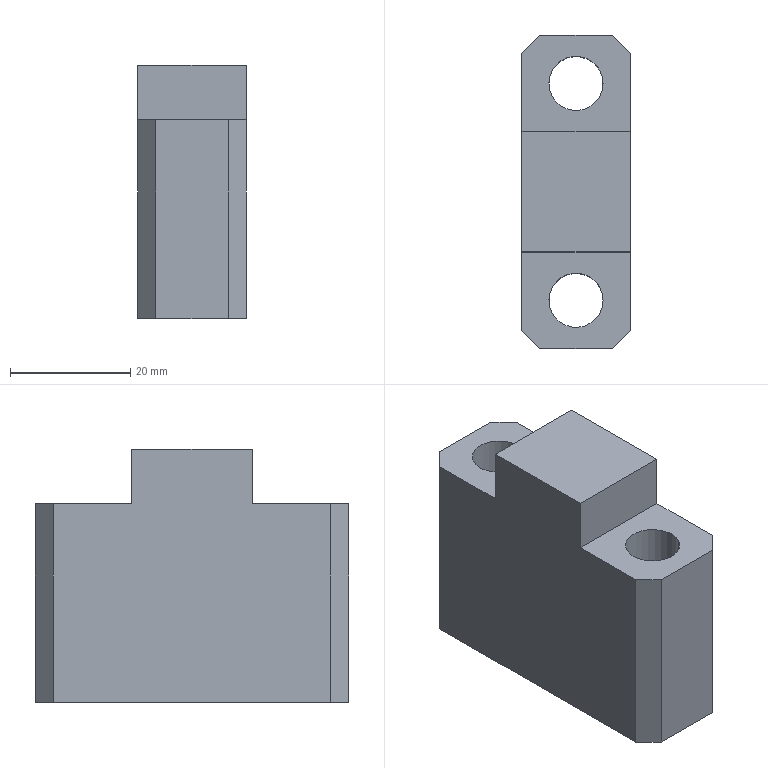Part | CATIA | 1 solid | 18 faces | box 18 x 52 x 42 mm | volume 29335 mm3 | plane 14 | cylinder 4 | commonest cylinder face diameters 9 x4
STEP:
#1=CARTESIAN_POINT('',(-1312.,219.5,-9.));
#2=VERTEX_POINT('',#1);
#3=CARTESIAN_POINT('',(-1312.,219.5,-42.));
#4=VERTEX_POINT('',#3);
#5=CARTESIAN_POINT('',(-1312.,219.5,-21.));
#6=DIRECTION('',(0.,0.,-1.));
#7=VECTOR('',#6,1.);
#8=LINE('',#5,#7);
#9=EDGE_CURVE('',#2,#4,#8,.T.);
#10=ORIENTED_EDGE('',*,*,#9,.T.);
#11=CARTESIAN_POINT('',(-1315.,222.5,-42.));
#12=VERTEX_POINT('',#11);
#13=CARTESIAN_POINT('',(-1313.5,221.,-42.));
#14=DIRECTION('',(-0.7071,0.7071,0.));
#15=VECTOR('',#14,1.);
#16=LINE('',#13,#15);
#17=EDGE_CURVE('',#4,#12,#16,.T.);
#18=ORIENTED_EDGE('',*,*,#17,.T.);
#19=CARTESIAN_POINT('',(-1315.,222.5,-9.));
#20=VERTEX_POINT('',#19);
#21=CARTESIAN_POINT('',(-1315.,222.5,-21.));
#22=DIRECTION('',(0.,0.,-1.));
#23=VECTOR('',#22,1.);
#24=LINE('',#21,#23);
#25=EDGE_CURVE('',#20,#12,#24,.T.);
#26=ORIENTED_EDGE('',*,*,#25,.F.);
#27=CARTESIAN_POINT('',(-1313.5,221.,-9.));
#28=DIRECTION('',(-0.7071,0.7071,0.));
#29=VECTOR('',#28,1.);
#30=LINE('',#27,#29);
#31=EDGE_CURVE('',#20,#2,#30,.F.);
#32=ORIENTED_EDGE('',*,*,#31,.T.);
#33=EDGE_LOOP('',(#10,#18,#26,#32));
#34=FACE_OUTER_BOUND('',#33,.T.);
#35=CARTESIAN_POINT('',(-1312.,219.5,8.4));
#36=DIRECTION('',(0.7071,0.7071,0.));
#37=DIRECTION('',(0.,0.,-1.));
#38=AXIS2_PLACEMENT_3D('',#35,#36,#37);
#39=PLANE('',#38);
#40=ADVANCED_FACE('',(#34),#39,.T.);
#41=CARTESIAN_POINT('',(-1330.,186.5,0.));
#42=VERTEX_POINT('',#41);
#43=CARTESIAN_POINT('',(-1312.,186.5,0.));
#44=VERTEX_POINT('',#43);
#45=CARTESIAN_POINT('',(-1321.,186.5,0.));
#46=DIRECTION('',(1.,0.,0.));
#47=VECTOR('',#46,1.);
#48=LINE('',#45,#47);
#49=EDGE_CURVE('',#42,#44,#48,.T.);
#50=ORIENTED_EDGE('',*,*,#49,.T.);
#51=CARTESIAN_POINT('',(-1312.,206.5,0.));
#52=VERTEX_POINT('',#51);
#53=CARTESIAN_POINT('',(-1312.,196.5,0.));
#54=DIRECTION('',(0.,1.,0.));
#55=VECTOR('',#54,1.);
#56=LINE('',#53,#55);
#57=EDGE_CURVE('',#44,#52,#56,.T.);
#58=ORIENTED_EDGE('',*,*,#57,.T.);
#59=CARTESIAN_POINT('',(-1330.,206.5,0.));
#60=VERTEX_POINT('',#59);
#61=CARTESIAN_POINT('',(-1321.,206.5,0.));
#62=DIRECTION('',(1.,0.,0.));
#63=VECTOR('',#62,1.);
#64=LINE('',#61,#63);
#65=EDGE_CURVE('',#60,#52,#64,.T.);
#66=ORIENTED_EDGE('',*,*,#65,.F.);
#67=CARTESIAN_POINT('',(-1330.,196.5,0.));
#68=DIRECTION('',(0.,-1.,0.));
#69=VECTOR('',#68,1.);
#70=LINE('',#67,#69);
#71=EDGE_CURVE('',#60,#42,#70,.T.);
#72=ORIENTED_EDGE('',*,*,#71,.T.);
#73=EDGE_LOOP('',(#50,#58,#66,#72));
#74=FACE_OUTER_BOUND('',#73,.T.);
#75=CARTESIAN_POINT('',(0.,0.,0.));
#76=DIRECTION('',(0.,0.,1.));
#77=DIRECTION('',(1.,0.,0.));
#78=AXIS2_PLACEMENT_3D('',#75,#76,#77);
#79=PLANE('',#78);
#80=ADVANCED_FACE('',(#74),#79,.T.);
#81=CARTESIAN_POINT('',(-1312.,186.5,-9.));
#82=VERTEX_POINT('',#81);
#83=CARTESIAN_POINT('',(-1312.,186.5,-4.5));
#84=DIRECTION('',(0.,0.,1.));
#85=VECTOR('',#84,1.);
#86=LINE('',#83,#85);
#87=EDGE_CURVE('',#82,#44,#86,.T.);
#88=ORIENTED_EDGE('',*,*,#87,.F.);
#89=CARTESIAN_POINT('',(-1312.,173.5,-9.));
#90=VERTEX_POINT('',#89);
#91=CARTESIAN_POINT('',(-1312.,180.,-9.));
#92=DIRECTION('',(0.,-1.,0.));
#93=VECTOR('',#92,1.);
#94=LINE('',#91,#93);
#95=EDGE_CURVE('',#82,#90,#94,.T.);
#96=ORIENTED_EDGE('',*,*,#95,.T.);
#97=CARTESIAN_POINT('',(-1312.,173.5,-42.));
#98=VERTEX_POINT('',#97);
#99=CARTESIAN_POINT('',(-1312.,173.5,-25.5));
#100=DIRECTION('',(0.,0.,1.));
#101=VECTOR('',#100,1.);
#102=LINE('',#99,#101);
#103=EDGE_CURVE('',#90,#98,#102,.F.);
#104=ORIENTED_EDGE('',*,*,#103,.T.);
#105=CARTESIAN_POINT('',(-1312.,196.5,-42.));
#106=DIRECTION('',(0.,1.,0.));
#107=VECTOR('',#106,1.);
#108=LINE('',#105,#107);
#109=EDGE_CURVE('',#98,#4,#108,.T.);
#110=ORIENTED_EDGE('',*,*,#109,.T.);
#111=ORIENTED_EDGE('',*,*,#9,.F.);
#112=CARTESIAN_POINT('',(-1312.,206.5,-9.));
#113=VERTEX_POINT('',#112);
#114=CARTESIAN_POINT('',(-1312.,213.,-9.));
#115=DIRECTION('',(0.,1.,0.));
#116=VECTOR('',#115,1.);
#117=LINE('',#114,#116);
#118=EDGE_CURVE('',#113,#2,#117,.T.);
#119=ORIENTED_EDGE('',*,*,#118,.F.);
#120=CARTESIAN_POINT('',(-1312.,206.5,-4.5));
#121=DIRECTION('',(0.,0.,1.));
#122=VECTOR('',#121,1.);
#123=LINE('',#120,#122);
#124=EDGE_CURVE('',#113,#52,#123,.T.);
#125=ORIENTED_EDGE('',*,*,#124,.T.);
#126=ORIENTED_EDGE('',*,*,#57,.F.);
#127=EDGE_LOOP('',(#88,#96,#104,#110,#111,#119,#125,#126));
#128=FACE_OUTER_BOUND('',#127,.T.);
#129=CARTESIAN_POINT('',(-1312.,170.5,0.));
#130=DIRECTION('',(-1.,0.,0.));
#131=DIRECTION('',(0.,1.,0.));
#132=AXIS2_PLACEMENT_3D('',#129,#130,#131);
#133=PLANE('',#132);
#134=ADVANCED_FACE('',(#128),#133,.F.);
#135=ORIENTED_EDGE('',*,*,#25,.T.);
#136=CARTESIAN_POINT('',(-1327.,222.5,-42.));
#137=VERTEX_POINT('',#136);
#138=CARTESIAN_POINT('',(-1321.,222.5,-42.));
#139=DIRECTION('',(1.,0.,0.));
#140=VECTOR('',#139,1.);
#141=LINE('',#138,#140);
#142=EDGE_CURVE('',#137,#12,#141,.T.);
#143=ORIENTED_EDGE('',*,*,#142,.F.);
#144=CARTESIAN_POINT('',(-1327.,222.5,-9.));
#145=VERTEX_POINT('',#144);
#146=CARTESIAN_POINT('',(-1327.,222.5,-25.5));
#147=DIRECTION('',(0.,0.,1.));
#148=VECTOR('',#147,1.);
#149=LINE('',#146,#148);
#150=EDGE_CURVE('',#145,#137,#149,.F.);
#151=ORIENTED_EDGE('',*,*,#150,.F.);
#152=CARTESIAN_POINT('',(-1321.,222.5,-9.));
#153=DIRECTION('',(1.,0.,0.));
#154=VECTOR('',#153,1.);
#155=LINE('',#152,#154);
#156=EDGE_CURVE('',#145,#20,#155,.T.);
#157=ORIENTED_EDGE('',*,*,#156,.T.);
#158=EDGE_LOOP('',(#135,#143,#151,#157));
#159=FACE_OUTER_BOUND('',#158,.T.);
#160=CARTESIAN_POINT('',(-1330.,222.5,0.));
#161=DIRECTION('',(0.,1.,0.));
#162=DIRECTION('',(1.,0.,0.));
#163=AXIS2_PLACEMENT_3D('',#160,#161,#162);
#164=PLANE('',#163);
#165=ADVANCED_FACE('',(#159),#164,.T.);
#166=CARTESIAN_POINT('',(-1315.,170.5,-9.));
#167=VERTEX_POINT('',#166);
#168=CARTESIAN_POINT('',(-1315.,170.5,-42.));
#169=VERTEX_POINT('',#168);
#170=CARTESIAN_POINT('',(-1315.,170.5,-21.));
#171=DIRECTION('',(0.,0.,1.));
#172=VECTOR('',#171,1.);
#173=LINE('',#170,#172);
#174=EDGE_CURVE('',#167,#169,#173,.F.);
#175=ORIENTED_EDGE('',*,*,#174,.T.);
#176=CARTESIAN_POINT('',(-1313.5,172.,-42.));
#177=DIRECTION('',(-0.7071,-0.7071,0.));
#178=VECTOR('',#177,1.);
#179=LINE('',#176,#178);
#180=EDGE_CURVE('',#169,#98,#179,.F.);
#181=ORIENTED_EDGE('',*,*,#180,.T.);
#182=ORIENTED_EDGE('',*,*,#103,.F.);
#183=CARTESIAN_POINT('',(-1313.5,172.,-9.));
#184=DIRECTION('',(-0.7071,-0.7071,0.));
#185=VECTOR('',#184,1.);
#186=LINE('',#183,#185);
#187=EDGE_CURVE('',#167,#90,#186,.F.);
#188=ORIENTED_EDGE('',*,*,#187,.F.);
#189=EDGE_LOOP('',(#175,#181,#182,#188));
#190=FACE_OUTER_BOUND('',#189,.T.);
#191=CARTESIAN_POINT('',(-1312.,173.5,-50.4));
#192=DIRECTION('',(0.7071,-0.7071,0.));
#193=DIRECTION('',(0.,0.,1.));
#194=AXIS2_PLACEMENT_3D('',#191,#192,#193);
#195=PLANE('',#194);
#196=ADVANCED_FACE('',(#190),#195,.T.);
#197=CARTESIAN_POINT('',(-1327.,170.5,-9.));
#198=VERTEX_POINT('',#197);
#199=CARTESIAN_POINT('',(-1327.,170.5,-42.));
#200=VERTEX_POINT('',#199);
#201=CARTESIAN_POINT('',(-1327.,170.5,-25.5));
#202=DIRECTION('',(0.,0.,-1.));
#203=VECTOR('',#202,1.);
#204=LINE('',#201,#203);
#205=EDGE_CURVE('',#198,#200,#204,.T.);
#206=ORIENTED_EDGE('',*,*,#205,.T.);
#207=CARTESIAN_POINT('',(-1321.,170.5,-42.));
#208=DIRECTION('',(-1.,0.,0.));
#209=VECTOR('',#208,1.);
#210=LINE('',#207,#209);
#211=EDGE_CURVE('',#169,#200,#210,.T.);
#212=ORIENTED_EDGE('',*,*,#211,.F.);
#213=ORIENTED_EDGE('',*,*,#174,.F.);
#214=CARTESIAN_POINT('',(-1321.,170.5,-9.));
#215=DIRECTION('',(-1.,0.,0.));
#216=VECTOR('',#215,1.);
#217=LINE('',#214,#216);
#218=EDGE_CURVE('',#167,#198,#217,.T.);
#219=ORIENTED_EDGE('',*,*,#218,.T.);
#220=EDGE_LOOP('',(#206,#212,#213,#219));
#221=FACE_OUTER_BOUND('',#220,.T.);
#222=CARTESIAN_POINT('',(-1312.,170.5,0.));
#223=DIRECTION('',(0.,-1.,0.));
#224=DIRECTION('',(-1.,0.,0.));
#225=AXIS2_PLACEMENT_3D('',#222,#223,#224);
#226=PLANE('',#225);
#227=ADVANCED_FACE('',(#221),#226,.T.);
#228=ORIENTED_EDGE('',*,*,#150,.T.);
#229=CARTESIAN_POINT('',(-1330.,219.5,-42.));
#230=VERTEX_POINT('',#229);
#231=CARTESIAN_POINT('',(-1328.5,221.,-42.));
#232=DIRECTION('',(0.7071,0.7071,0.));
#233=VECTOR('',#232,1.);
#234=LINE('',#231,#233);
#235=EDGE_CURVE('',#137,#230,#234,.F.);
#236=ORIENTED_EDGE('',*,*,#235,.T.);
#237=CARTESIAN_POINT('',(-1330.,219.5,-9.));
#238=VERTEX_POINT('',#237);
#239=CARTESIAN_POINT('',(-1330.,219.5,-21.));
#240=DIRECTION('',(0.,0.,1.));
#241=VECTOR('',#240,1.);
#242=LINE('',#239,#241);
#243=EDGE_CURVE('',#238,#230,#242,.F.);
#244=ORIENTED_EDGE('',*,*,#243,.F.);
#245=CARTESIAN_POINT('',(-1328.5,221.,-9.));
#246=DIRECTION('',(0.7071,0.7071,0.));
#247=VECTOR('',#246,1.);
#248=LINE('',#245,#247);
#249=EDGE_CURVE('',#145,#238,#248,.F.);
#250=ORIENTED_EDGE('',*,*,#249,.F.);
#251=EDGE_LOOP('',(#228,#236,#244,#250));
#252=FACE_OUTER_BOUND('',#251,.T.);
#253=CARTESIAN_POINT('',(-1330.,219.5,-50.4));
#254=DIRECTION('',(-0.7071,0.7071,0.));
#255=DIRECTION('',(0.,0.,1.));
#256=AXIS2_PLACEMENT_3D('',#253,#254,#255);
#257=PLANE('',#256);
#258=ADVANCED_FACE('',(#252),#257,.T.);
#259=ORIENTED_EDGE('',*,*,#71,.F.);
#260=CARTESIAN_POINT('',(-1330.,206.5,-9.));
#261=VERTEX_POINT('',#260);
#262=CARTESIAN_POINT('',(-1330.,206.5,-4.5));
#263=DIRECTION('',(0.,0.,1.));
#264=VECTOR('',#263,1.);
#265=LINE('',#262,#264);
#266=EDGE_CURVE('',#261,#60,#265,.T.);
#267=ORIENTED_EDGE('',*,*,#266,.F.);
#268=CARTESIAN_POINT('',(-1330.,213.,-9.));
#269=DIRECTION('',(0.,1.,0.));
#270=VECTOR('',#269,1.);
#271=LINE('',#268,#270);
#272=EDGE_CURVE('',#261,#238,#271,.T.);
#273=ORIENTED_EDGE('',*,*,#272,.T.);
#274=ORIENTED_EDGE('',*,*,#243,.T.);
#275=CARTESIAN_POINT('',(-1330.,173.5,-42.));
#276=VERTEX_POINT('',#275);
#277=CARTESIAN_POINT('',(-1330.,196.5,-42.));
#278=DIRECTION('',(0.,-1.,0.));
#279=VECTOR('',#278,1.);
#280=LINE('',#277,#279);
#281=EDGE_CURVE('',#230,#276,#280,.T.);
#282=ORIENTED_EDGE('',*,*,#281,.T.);
#283=CARTESIAN_POINT('',(-1330.,173.5,-9.));
#284=VERTEX_POINT('',#283);
#285=CARTESIAN_POINT('',(-1330.,173.5,-25.5));
#286=DIRECTION('',(0.,0.,-1.));
#287=VECTOR('',#286,1.);
#288=LINE('',#285,#287);
#289=EDGE_CURVE('',#284,#276,#288,.T.);
#290=ORIENTED_EDGE('',*,*,#289,.F.);
#291=CARTESIAN_POINT('',(-1330.,186.5,-9.));
#292=VERTEX_POINT('',#291);
#293=CARTESIAN_POINT('',(-1330.,180.,-9.));
#294=DIRECTION('',(0.,-1.,0.));
#295=VECTOR('',#294,1.);
#296=LINE('',#293,#295);
#297=EDGE_CURVE('',#292,#284,#296,.T.);
#298=ORIENTED_EDGE('',*,*,#297,.F.);
#299=CARTESIAN_POINT('',(-1330.,186.5,-4.5));
#300=DIRECTION('',(0.,0.,1.));
#301=VECTOR('',#300,1.);
#302=LINE('',#299,#301);
#303=EDGE_CURVE('',#292,#42,#302,.T.);
#304=ORIENTED_EDGE('',*,*,#303,.T.);
#305=EDGE_LOOP('',(#259,#267,#273,#274,#282,#290,#298,#304));
#306=FACE_OUTER_BOUND('',#305,.T.);
#307=CARTESIAN_POINT('',(-1330.,222.5,0.));
#308=DIRECTION('',(1.,0.,0.));
#309=DIRECTION('',(0.,-1.,0.));
#310=AXIS2_PLACEMENT_3D('',#307,#308,#309);
#311=PLANE('',#310);
#312=ADVANCED_FACE('',(#306),#311,.F.);
#313=ORIENTED_EDGE('',*,*,#289,.T.);
#314=CARTESIAN_POINT('',(-1328.5,172.,-42.));
#315=DIRECTION('',(0.7071,-0.7071,0.));
#316=VECTOR('',#315,1.);
#317=LINE('',#314,#316);
#318=EDGE_CURVE('',#276,#200,#317,.T.);
#319=ORIENTED_EDGE('',*,*,#318,.T.);
#320=ORIENTED_EDGE('',*,*,#205,.F.);
#321=CARTESIAN_POINT('',(-1328.5,172.,-9.));
#322=DIRECTION('',(0.7071,-0.7071,0.));
#323=VECTOR('',#322,1.);
#324=LINE('',#321,#323);
#325=EDGE_CURVE('',#198,#284,#324,.F.);
#326=ORIENTED_EDGE('',*,*,#325,.T.);
#327=EDGE_LOOP('',(#313,#319,#320,#326));
#328=FACE_OUTER_BOUND('',#327,.T.);
#329=CARTESIAN_POINT('',(-1330.,173.5,8.4));
#330=DIRECTION('',(-0.7071,-0.7071,0.));
#331=DIRECTION('',(0.,0.,-1.));
#332=AXIS2_PLACEMENT_3D('',#329,#330,#331);
#333=PLANE('',#332);
#334=ADVANCED_FACE('',(#328),#333,.T.);
#335=ORIENTED_EDGE('',*,*,#87,.T.);
#336=ORIENTED_EDGE('',*,*,#49,.F.);
#337=ORIENTED_EDGE('',*,*,#303,.F.);
#338=CARTESIAN_POINT('',(-1321.,186.5,-9.));
#339=DIRECTION('',(1.,0.,0.));
#340=VECTOR('',#339,1.);
#341=LINE('',#338,#340);
#342=EDGE_CURVE('',#82,#292,#341,.F.);
#343=ORIENTED_EDGE('',*,*,#342,.F.);
#344=EDGE_LOOP('',(#335,#336,#337,#343));
#345=FACE_OUTER_BOUND('',#344,.T.);
#346=CARTESIAN_POINT('',(-1405.,186.5,0.));
#347=DIRECTION('',(0.,1.,0.));
#348=DIRECTION('',(1.,0.,0.));
#349=AXIS2_PLACEMENT_3D('',#346,#347,#348);
#350=PLANE('',#349);
#351=ADVANCED_FACE('',(#345),#350,.F.);
#352=ORIENTED_EDGE('',*,*,#266,.T.);
#353=ORIENTED_EDGE('',*,*,#65,.T.);
#354=ORIENTED_EDGE('',*,*,#124,.F.);
#355=CARTESIAN_POINT('',(-1321.,206.5,-9.));
#356=DIRECTION('',(-1.,0.,0.));
#357=VECTOR('',#356,1.);
#358=LINE('',#355,#357);
#359=EDGE_CURVE('',#261,#113,#358,.F.);
#360=ORIENTED_EDGE('',*,*,#359,.F.);
#361=EDGE_LOOP('',(#352,#353,#354,#360));
#362=FACE_OUTER_BOUND('',#361,.T.);
#363=CARTESIAN_POINT('',(-1159.802,206.5,0.));
#364=DIRECTION('',(0.,-1.,0.));
#365=DIRECTION('',(-1.,0.,0.));
#366=AXIS2_PLACEMENT_3D('',#363,#364,#365);
#367=PLANE('',#366);
#368=ADVANCED_FACE('',(#362),#367,.F.);
#369=ORIENTED_EDGE('',*,*,#359,.T.);
#370=ORIENTED_EDGE('',*,*,#118,.T.);
#371=ORIENTED_EDGE('',*,*,#31,.F.);
#372=ORIENTED_EDGE('',*,*,#156,.F.);
#373=ORIENTED_EDGE('',*,*,#249,.T.);
#374=ORIENTED_EDGE('',*,*,#272,.F.);
#375=EDGE_LOOP('',(#369,#370,#371,#372,#373,#374));
#376=FACE_OUTER_BOUND('',#375,.T.);
#377=CARTESIAN_POINT('',(-1324.949,216.657,-9.));
#378=VERTEX_POINT('',#377);
#379=CARTESIAN_POINT('',(-1317.051,212.343,-9.));
#380=VERTEX_POINT('',#379);
#381=CARTESIAN_POINT('',(-1321.,214.5,-9.));
#382=DIRECTION('',(0.,0.,1.));
#383=AXIS2_PLACEMENT_3D('',#381,#382,$);
#384=CIRCLE('',#383,4.5);
#385=EDGE_CURVE('',#378,#380,#384,.T.);
#386=ORIENTED_EDGE('',*,*,#385,.F.);
#387=CARTESIAN_POINT('',(-1321.,214.5,-9.));
#388=DIRECTION('',(0.,0.,1.));
#389=AXIS2_PLACEMENT_3D('',#387,#388,$);
#390=CIRCLE('',#389,4.5);
#391=EDGE_CURVE('',#380,#378,#390,.T.);
#392=ORIENTED_EDGE('',*,*,#391,.F.);
#393=EDGE_LOOP('',(#386,#392));
#394=FACE_BOUND('',#393,.T.);
#395=CARTESIAN_POINT('',(0.,0.,-9.));
#396=DIRECTION('',(0.,0.,1.));
#397=DIRECTION('',(1.,0.,0.));
#398=AXIS2_PLACEMENT_3D('',#395,#396,#397);
#399=PLANE('',#398);
#400=ADVANCED_FACE('',(#376,#394),#399,.T.);
#401=ORIENTED_EDGE('',*,*,#342,.T.);
#402=ORIENTED_EDGE('',*,*,#297,.T.);
#403=ORIENTED_EDGE('',*,*,#325,.F.);
#404=ORIENTED_EDGE('',*,*,#218,.F.);
#405=ORIENTED_EDGE('',*,*,#187,.T.);
#406=ORIENTED_EDGE('',*,*,#95,.F.);
#407=EDGE_LOOP('',(#401,#402,#403,#404,#405,#406));
#408=FACE_OUTER_BOUND('',#407,.T.);
#409=CARTESIAN_POINT('',(-1324.949,180.657,-9.));
#410=VERTEX_POINT('',#409);
#411=CARTESIAN_POINT('',(-1317.051,176.343,-9.));
#412=VERTEX_POINT('',#411);
#413=CARTESIAN_POINT('',(-1321.,178.5,-9.));
#414=DIRECTION('',(0.,0.,1.));
#415=AXIS2_PLACEMENT_3D('',#413,#414,$);
#416=CIRCLE('',#415,4.5);
#417=EDGE_CURVE('',#410,#412,#416,.T.);
#418=ORIENTED_EDGE('',*,*,#417,.F.);
#419=CARTESIAN_POINT('',(-1321.,178.5,-9.));
#420=DIRECTION('',(0.,0.,1.));
#421=AXIS2_PLACEMENT_3D('',#419,#420,$);
#422=CIRCLE('',#421,4.5);
#423=EDGE_CURVE('',#412,#410,#422,.T.);
#424=ORIENTED_EDGE('',*,*,#423,.F.);
#425=EDGE_LOOP('',(#418,#424));
#426=FACE_BOUND('',#425,.T.);
#427=ADVANCED_FACE('',(#408,#426),#399,.T.);
#428=ORIENTED_EDGE('',*,*,#17,.F.);
#429=ORIENTED_EDGE('',*,*,#109,.F.);
#430=ORIENTED_EDGE('',*,*,#180,.F.);
#431=ORIENTED_EDGE('',*,*,#211,.T.);
#432=ORIENTED_EDGE('',*,*,#318,.F.);
#433=ORIENTED_EDGE('',*,*,#281,.F.);
#434=ORIENTED_EDGE('',*,*,#235,.F.);
#435=ORIENTED_EDGE('',*,*,#142,.T.);
#436=EDGE_LOOP('',(#428,#429,#430,#431,#432,#433,#434,#435));
#437=FACE_OUTER_BOUND('',#436,.T.);
#438=CARTESIAN_POINT('',(-1324.949,180.657,-42.));
#439=VERTEX_POINT('',#438);
#440=CARTESIAN_POINT('',(-1317.051,176.343,-42.));
#441=VERTEX_POINT('',#440);
#442=CARTESIAN_POINT('',(-1321.,178.5,-42.));
#443=DIRECTION('',(0.,0.,1.));
#444=AXIS2_PLACEMENT_3D('',#442,#443,$);
#445=CIRCLE('',#444,4.5);
#446=EDGE_CURVE('',#439,#441,#445,.T.);
#447=ORIENTED_EDGE('',*,*,#446,.T.);
#448=CARTESIAN_POINT('',(-1321.,178.5,-42.));
#449=DIRECTION('',(0.,0.,1.));
#450=AXIS2_PLACEMENT_3D('',#448,#449,$);
#451=CIRCLE('',#450,4.5);
#452=EDGE_CURVE('',#441,#439,#451,.T.);
#453=ORIENTED_EDGE('',*,*,#452,.T.);
#454=EDGE_LOOP('',(#447,#453));
#455=FACE_BOUND('',#454,.T.);
#456=CARTESIAN_POINT('',(-1324.949,216.657,-42.));
#457=VERTEX_POINT('',#456);
#458=CARTESIAN_POINT('',(-1317.051,212.343,-42.));
#459=VERTEX_POINT('',#458);
#460=CARTESIAN_POINT('',(-1321.,214.5,-42.));
#461=DIRECTION('',(0.,0.,1.));
#462=AXIS2_PLACEMENT_3D('',#460,#461,$);
#463=CIRCLE('',#462,4.5);
#464=EDGE_CURVE('',#457,#459,#463,.T.);
#465=ORIENTED_EDGE('',*,*,#464,.T.);
#466=CARTESIAN_POINT('',(-1321.,214.5,-42.));
#467=DIRECTION('',(0.,0.,1.));
#468=AXIS2_PLACEMENT_3D('',#466,#467,$);
#469=CIRCLE('',#468,4.5);
#470=EDGE_CURVE('',#459,#457,#469,.T.);
#471=ORIENTED_EDGE('',*,*,#470,.T.);
#472=EDGE_LOOP('',(#465,#471));
#473=FACE_BOUND('',#472,.T.);
#474=CARTESIAN_POINT('',(0.,0.,-42.));
#475=DIRECTION('',(0.,0.,1.));
#476=DIRECTION('',(1.,0.,0.));
#477=AXIS2_PLACEMENT_3D('',#474,#475,#476);
#478=PLANE('',#477);
#479=ADVANCED_FACE('',(#437,#455,#473),#478,.F.);
#480=ORIENTED_EDGE('',*,*,#423,.T.);
#481=CARTESIAN_POINT('',(-1324.949,180.657,-21.));
#482=DIRECTION('',(0.,0.,-1.));
#483=VECTOR('',#482,1.);
#484=LINE('',#481,#483);
#485=EDGE_CURVE('',#439,#410,#484,.F.);
#486=ORIENTED_EDGE('',*,*,#485,.F.);
#487=ORIENTED_EDGE('',*,*,#452,.F.);
#488=CARTESIAN_POINT('',(-1317.051,176.343,-21.));
#489=DIRECTION('',(0.,0.,-1.));
#490=VECTOR('',#489,1.);
#491=LINE('',#488,#490);
#492=EDGE_CURVE('',#441,#412,#491,.F.);
#493=ORIENTED_EDGE('',*,*,#492,.T.);
#494=EDGE_LOOP('',(#480,#486,#487,#493));
#495=FACE_OUTER_BOUND('',#494,.T.);
#496=CARTESIAN_POINT('',(-1321.,178.5,-0.1));
#497=DIRECTION('',(0.,0.,-1.));
#498=DIRECTION('',(0.8776,-0.4794,0.));
#499=AXIS2_PLACEMENT_3D('',#496,#497,#498);
#500=CYLINDRICAL_SURFACE('',#499,4.5);
#501=ADVANCED_FACE('',(#495),#500,.F.);
#502=ORIENTED_EDGE('',*,*,#417,.T.);
#503=ORIENTED_EDGE('',*,*,#492,.F.);
#504=ORIENTED_EDGE('',*,*,#446,.F.);
#505=ORIENTED_EDGE('',*,*,#485,.T.);
#506=EDGE_LOOP('',(#502,#503,#504,#505));
#507=FACE_OUTER_BOUND('',#506,.T.);
#508=ADVANCED_FACE('',(#507),#500,.F.);
#509=ORIENTED_EDGE('',*,*,#391,.T.);
#510=CARTESIAN_POINT('',(-1324.949,216.657,-21.));
#511=DIRECTION('',(0.,0.,-1.));
#512=VECTOR('',#511,1.);
#513=LINE('',#510,#512);
#514=EDGE_CURVE('',#457,#378,#513,.F.);
#515=ORIENTED_EDGE('',*,*,#514,.F.);
#516=ORIENTED_EDGE('',*,*,#470,.F.);
#517=CARTESIAN_POINT('',(-1317.051,212.343,-21.));
#518=DIRECTION('',(0.,0.,-1.));
#519=VECTOR('',#518,1.);
#520=LINE('',#517,#519);
#521=EDGE_CURVE('',#459,#380,#520,.F.);
#522=ORIENTED_EDGE('',*,*,#521,.T.);
#523=EDGE_LOOP('',(#509,#515,#516,#522));
#524=FACE_OUTER_BOUND('',#523,.T.);
#525=CARTESIAN_POINT('',(-1321.,214.5,-0.1));
#526=DIRECTION('',(0.,0.,-1.));
#527=DIRECTION('',(0.8776,-0.4794,0.));
#528=AXIS2_PLACEMENT_3D('',#525,#526,#527);
#529=CYLINDRICAL_SURFACE('',#528,4.5);
#530=ADVANCED_FACE('',(#524),#529,.F.);
#531=ORIENTED_EDGE('',*,*,#385,.T.);
#532=ORIENTED_EDGE('',*,*,#521,.F.);
#533=ORIENTED_EDGE('',*,*,#464,.F.);
#534=ORIENTED_EDGE('',*,*,#514,.T.);
#535=EDGE_LOOP('',(#531,#532,#533,#534));
#536=FACE_OUTER_BOUND('',#535,.T.);
#537=ADVANCED_FACE('',(#536),#529,.F.);
#538=CLOSED_SHELL('',(#40,#80,#134,#165,#196,#227,#258,#312,#334,#351,#368,#400,#427,#479,#501,#508,#530,#537));
#539=MANIFOLD_SOLID_BREP('',#538);
#540=(LENGTH_UNIT()NAMED_UNIT(*)SI_UNIT(.MILLI.,.METRE.));
#541=UNCERTAINTY_MEASURE_WITH_UNIT(LENGTH_MEASURE(0.005),#540,'','');
#542=(NAMED_UNIT(*)PLANE_ANGLE_UNIT()SI_UNIT($,.RADIAN.));
#543=(NAMED_UNIT(*)SI_UNIT($,.STERADIAN.)SOLID_ANGLE_UNIT());
#544=(GEOMETRIC_REPRESENTATION_CONTEXT(3)GLOBAL_UNCERTAINTY_ASSIGNED_CONTEXT((#541))GLOBAL_UNIT_ASSIGNED_CONTEXT((#540,#542,#543))REPRESENTATION_CONTEXT('',''));
#545=ADVANCED_BREP_SHAPE_REPRESENTATION('',(#539),#544);